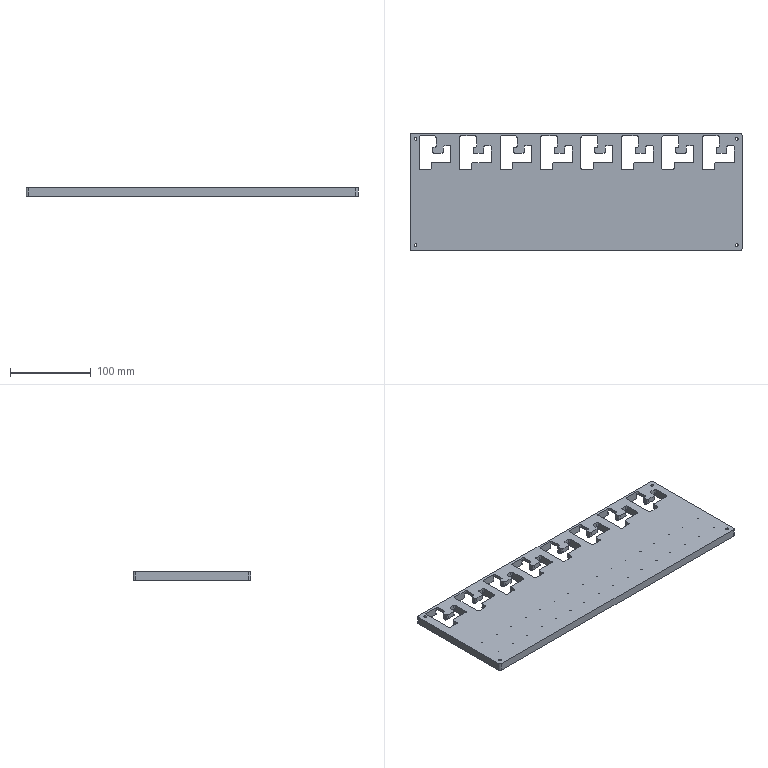CAM job | NX | 3-axis milling, drilling | part box 410 x 145 x 10 mm | stock box 414 x 145 x 11 mm
Tools:
number,name,description,diameter,corner_radius,flute_length,length,flutes
1,D63,Milling Tool-5 Parameters,63.0,0.0,50.0,75.0,2
7,D6A45,Milling Tool-5 Parameters,6.0,0.0,3.0,3.0,2
10,D10,Milling Tool-5 Parameters,10.0,0.0,50.0,75.0,2
6,D6,Milling Tool-5 Parameters,6.0,0.0,50.0,75.0,2
3,D3,Milling Tool-5 Parameters,3.0,0.0,50.0,75.0,2
13,3.2ZT,Drilling Tool,3.2,0.0,35.0,50.0,2
15,1.59ZT,Drilling Tool,1.59,0.0,35.0,50.0,2
16,D1.55YD,Thread Mill,1.55,0.0,0.4,50.0,2
11,2.05ZT,Drilling Tool,2.05,0.0,35.0,50.0,2
12,D1.96YD,Thread Mill,1.96,0.0,0.45,50.0,2
14,1.05ZT,Drilling Tool,1.05,0.0,35.0,50.0,2
20,D1.5,Milling Tool-5 Parameters,1.5,0.0,50.0,75.0,2
21,D0.7,Milling Tool-5 Parameters,0.7,0.0,50.0,75.0,2
22,D3A45,Milling Tool-5 Parameters,3.0,0.0,1.5,1.5,2
Operations:
program,operation,operation_type,tool,method,geometry_group,spindle_rpm,surface_speed,feed_per_tooth,feed_cut,feed_plunge,cut_length_mm,path_length_mm,cut_time_min,machine_time_min
1,FLOOR_WALL,VolumeBased25DMillingOperation,D63,METHOD,A,6500.0,1286.0,0.0962,1250.0,100.0,2516.797,2570.797,2.013,2.019
1,ZLEVEL_PROFILE,ZLevelMilling,D10,METHOD,A,9500.0,298.0,0.1316,2500.0,100.0,3449.985,4039.081,1.38,1.439
1,ZLEVEL_PROFILE_COPY,ZLevelMilling,D10,METHOD,A,9500.0,298.0,0.0526,1000.0,100.0,351.907,902.609,0.3519,0.407
1,CAVITY_MILL,CavityMilling,D10,METHOD,A,9500.0,298.0,0.1579,3000.0,1000.0,41832.07,51906.799,17.881,18.888
1,CAVITY_MILL_COPY,CavityMilling,D6,METHOD,A,9500.0,179.0,0.0868,1650.0,1000.0,16973.893,40229.096,12.033,14.358
1,DRILLING,Operation,D6A45,METHOD,A,5000.0,94.0,0.025,250.0,0.0,300.0,2462.83,1.2,1.416
1,DRILLING_COPY,Operation,3.2ZT,METHOD,A,2000.0,20.0,0.0375,150.0,0.0,47.846,830.271,0.319,0.3972
1,DRILLING_COPY_COPY,Operation,1.59ZT,METHOD,A,2000.0,9.0,0.0375,150.0,0.0,407.286,1804.336,2.715,2.855
1,刀补16,ThreadMilling,D1.55YD,METHOD,A,6500.0,31.0,0.0769,1000.0,100.0,1991.399,9539.399,1.991,2.746
1,DRILLING_COPY_COPY_COPY,Operation,2.05ZT,METHOD,A,1397.0,9.0,0.0537,150.0,0.0,264.0,1507.731,1.76,1.884
1,刀补16_COPY,ThreadMilling,D1.96YD,METHOD,A,6500.0,31.0,0.0769,1000.0,100.0,1695.804,7426.129,1.696,2.269
1,DRILLING_COPY_COPY_COPY_COPY,Operation,1.05ZT,METHOD,A,1397.0,9.0,0.0537,150.0,0.0,72.0,579.629,0.48,0.5308
1,CAVITY_MILL_COPY_COPY,CavityMilling,D3,METHOD,A,9500.0,89.0,0.0632,1200.0,1000.0,28298.901,64418.396,24.284,27.896
1,HOLE_MILLING,CylinderMilling,D3,METHOD,A,9500.0,89.0,0.0658,1250.0,100.0,279.729,536.729,0.2238,0.2495
1,FLOOR_WALL_1,VolumeBased25DMillingOperation,D3,METHOD,A,9500.0,89.0,0.0579,1100.0,100.0,21444.053,34396.697,19.495,20.79
1,FLOOR_WALL_1_COPY,VolumeBased25DMillingOperation,D3,METHOD,A,9500.0,89.0,0.0579,1100.0,100.0,14473.051,22391.138,13.157,13.949
1,ZLEVEL_PROFILE_1,ZLevelMilling,D3,METHOD,A,9500.0,89.0,0.0526,1000.0,100.0,1399.137,3373.149,1.399,1.597
1,CAVITY_MILL_COPY_COPY_COPY,CavityMilling,D1.5,METHOD,A,9500.0,44.0,0.0526,1000.0,1000.0,14388.256,50228.096,14.388,17.972
1,CAVITY_MILL_COPY_COPY_COPY_COPY,CavityMilling,D0.7,METHOD,A,9500.0,20.0,0.0447,850.0,850.0,2379.436,3588.679,2.799,2.92
1,ZLEVEL_PROFILE_2,ZLevelMilling,D6A45,METHOD,A,9500.0,179.0,0.0658,1250.0,100.0,4380.227,7550.5,3.504,3.821
1,ZLEVEL_PROFILE_2_COPY,ZLevelMilling,D6A45,METHOD,A,9500.0,179.0,0.0658,1250.0,100.0,954.145,4090.008,0.7633,1.077
1,ZLEVEL_PROFILE_2_COPY_COPY,ZLevelMilling,D6A45,METHOD,A,9500.0,179.0,0.0658,1250.0,100.0,915.109,3472.159,0.7321,0.9878
1,ZLEVEL_PROFILE_2_COPY_COPY_1,ZLevelMilling,D3A45,METHOD,A,9500.0,179.0,0.0658,1250.0,100.0,313.004,1011.317,0.2504,0.3202
1,ZLEVEL_PROFILE_2_COPY_COPY_1_COPY,ZLevelMilling,D3A45,METHOD,A,9500.0,179.0,0.0658,1250.0,100.0,313.004,1011.317,0.2504,0.3202
1,ZLEVEL_PROFILE_2_COPY_COPY_1_COPY_1,ZLevelMilling,D3A45,METHOD,A,9500.0,179.0,0.0658,1250.0,100.0,313.004,1011.317,0.2504,0.3202
1,ZLEVEL_PROFILE_2_COPY_COPY_1_COPY_2,ZLevelMilling,D3A45,METHOD,A,9500.0,179.0,0.0658,1250.0,100.0,313.004,1011.317,0.2504,0.3202
1,ZLEVEL_PROFILE_2_COPY_COPY_1_COPY_3,ZLevelMilling,D3A45,METHOD,A,9500.0,179.0,0.0658,1250.0,100.0,313.004,1011.317,0.2504,0.3202
1,ZLEVEL_PROFILE_2_COPY_COPY_1_COPY_4,ZLevelMilling,D3A45,METHOD,A,9500.0,179.0,0.0658,1250.0,100.0,313.004,1011.317,0.2504,0.3202
1,ZLEVEL_PROFILE_2_COPY_COPY_1_COPY_5,ZLevelMilling,D3A45,METHOD,A,9500.0,179.0,0.0658,1250.0,100.0,313.004,1011.317,0.2504,0.3202
1,ZLEVEL_PROFILE_2_COPY_COPY_1_COPY_6,ZLevelMilling,D3A45,METHOD,A,9500.0,179.0,0.0658,1250.0,100.0,313.004,1011.317,0.2504,0.3202
1,刀补3,ZLevelMilling,D3,METHOD,A,9500.0,89.0,0.0526,1000.0,100.0,542.736,2869.285,0.5427,0.7754
2,ZLEVEL_PROFILE_2_COPY_1,ZLevelMilling,D6A45,METHOD,B,9500.0,179.0,0.0658,1250.0,100.0,2592.362,5497.267,2.074,2.364